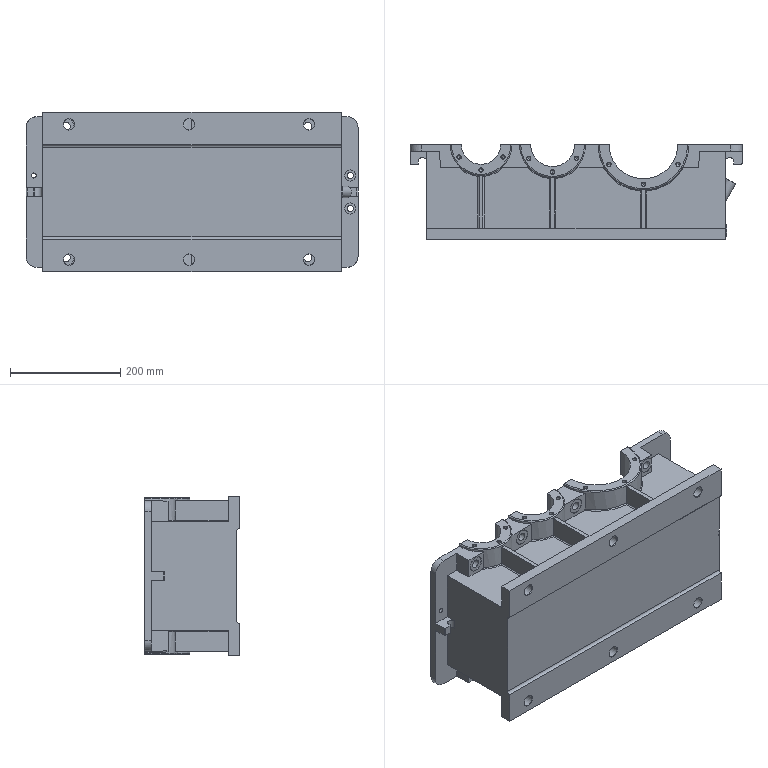Part | NX | 1 solid | 280 faces | box 603 x 172 x 290 mm | volume 5155522 mm3 | plane 105 | cylinder 96 | cone 52 | torus 17 | spline 6 | sphere 4 | commonest cylinder face diameters 4 x21 6.8 x18 15 x10 28.25 x8 20 x6 36 x6